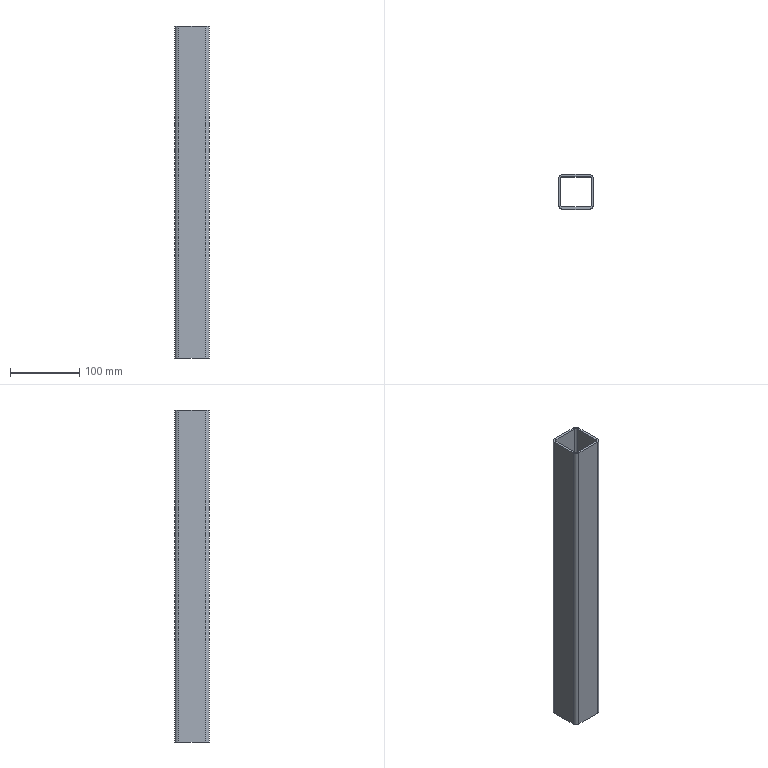Part | SolidWorks | features WeldMemberFeat 1, WeldmentFeature 1 | 1 solid | 18 faces | box 50 x 50 x 480 mm | volume 259595 mm3 | plane 10 | cylinder 8 | commonest cylinder face diameters 6 x4 12 x4
STEP:
#1=CARTESIAN_POINT('',(-25.,19.,0.));
#2=VERTEX_POINT('',#1);
#3=CARTESIAN_POINT('',(-19.,25.,0.));
#4=VERTEX_POINT('',#3);
#5=CARTESIAN_POINT('',(-19.,19.,0.));
#6=DIRECTION('',(0.,0.,-1.));
#7=DIRECTION('',(-1.,0.,0.));
#8=AXIS2_PLACEMENT_3D('',#5,#6,#7);
#9=CIRCLE('',#8,6.);
#10=EDGE_CURVE('',#2,#4,#9,.T.);
#11=ORIENTED_EDGE('',*,*,#10,.T.);
#12=CARTESIAN_POINT('',(-19.,25.,-480.));
#13=VERTEX_POINT('',#12);
#14=CARTESIAN_POINT('',(-19.,25.,-480.));
#15=DIRECTION('',(0.,0.,1.));
#16=VECTOR('',#15,1000.);
#17=LINE('',#14,#16);
#18=EDGE_CURVE('',#13,#4,#17,.T.);
#19=ORIENTED_EDGE('',*,*,#18,.F.);
#20=CARTESIAN_POINT('',(-25.,19.,-480.));
#21=VERTEX_POINT('',#20);
#22=CARTESIAN_POINT('',(-19.,19.,-480.));
#23=DIRECTION('',(0.,0.,-1.));
#24=DIRECTION('',(-1.,0.,0.));
#25=AXIS2_PLACEMENT_3D('',#22,#23,#24);
#26=CIRCLE('',#25,6.);
#27=EDGE_CURVE('',#21,#13,#26,.T.);
#28=ORIENTED_EDGE('',*,*,#27,.F.);
#29=CARTESIAN_POINT('',(-25.,19.,-480.));
#30=DIRECTION('',(0.,0.,1.));
#31=VECTOR('',#30,1000.);
#32=LINE('',#29,#31);
#33=EDGE_CURVE('',#21,#2,#32,.T.);
#34=ORIENTED_EDGE('',*,*,#33,.T.);
#35=EDGE_LOOP('',(#11,#19,#28,#34));
#36=FACE_OUTER_BOUND('',#35,.T.);
#37=CARTESIAN_POINT('',(-19.,19.,-480.));
#38=DIRECTION('',(0.,0.,1.));
#39=DIRECTION('',(1.,0.,0.));
#40=AXIS2_PLACEMENT_3D('',#37,#38,#39);
#41=CYLINDRICAL_SURFACE('',#40,6.);
#42=ADVANCED_FACE('',(#36),#41,.T.);
#43=CARTESIAN_POINT('',(19.,25.,0.));
#44=VERTEX_POINT('',#43);
#45=CARTESIAN_POINT('',(-19.,25.,0.));
#46=DIRECTION('',(1.,0.,0.));
#47=VECTOR('',#46,1000.);
#48=LINE('',#45,#47);
#49=EDGE_CURVE('',#4,#44,#48,.T.);
#50=ORIENTED_EDGE('',*,*,#49,.T.);
#51=CARTESIAN_POINT('',(19.,25.,-480.));
#52=VERTEX_POINT('',#51);
#53=CARTESIAN_POINT('',(19.,25.,-480.));
#54=DIRECTION('',(0.,0.,1.));
#55=VECTOR('',#54,1000.);
#56=LINE('',#53,#55);
#57=EDGE_CURVE('',#52,#44,#56,.T.);
#58=ORIENTED_EDGE('',*,*,#57,.F.);
#59=CARTESIAN_POINT('',(-19.,25.,-480.));
#60=DIRECTION('',(1.,0.,0.));
#61=VECTOR('',#60,1000.);
#62=LINE('',#59,#61);
#63=EDGE_CURVE('',#13,#52,#62,.T.);
#64=ORIENTED_EDGE('',*,*,#63,.F.);
#65=ORIENTED_EDGE('',*,*,#18,.T.);
#66=EDGE_LOOP('',(#50,#58,#64,#65));
#67=FACE_OUTER_BOUND('',#66,.T.);
#68=CARTESIAN_POINT('',(-19.,25.,-480.));
#69=DIRECTION('',(0.,-1.,0.));
#70=DIRECTION('',(0.,0.,-1.));
#71=AXIS2_PLACEMENT_3D('',#68,#69,#70);
#72=PLANE('',#71);
#73=ADVANCED_FACE('',(#67),#72,.F.);
#74=CARTESIAN_POINT('',(25.,19.,0.));
#75=VERTEX_POINT('',#74);
#76=CARTESIAN_POINT('',(19.,19.,0.));
#77=DIRECTION('',(0.,0.,-1.));
#78=DIRECTION('',(-1.,0.,0.));
#79=AXIS2_PLACEMENT_3D('',#76,#77,#78);
#80=CIRCLE('',#79,6.);
#81=EDGE_CURVE('',#44,#75,#80,.T.);
#82=ORIENTED_EDGE('',*,*,#81,.T.);
#83=CARTESIAN_POINT('',(25.,19.,-480.));
#84=VERTEX_POINT('',#83);
#85=CARTESIAN_POINT('',(25.,19.,-480.));
#86=DIRECTION('',(0.,0.,1.));
#87=VECTOR('',#86,1000.);
#88=LINE('',#85,#87);
#89=EDGE_CURVE('',#84,#75,#88,.T.);
#90=ORIENTED_EDGE('',*,*,#89,.F.);
#91=CARTESIAN_POINT('',(19.,19.,-480.));
#92=DIRECTION('',(0.,0.,-1.));
#93=DIRECTION('',(-1.,0.,0.));
#94=AXIS2_PLACEMENT_3D('',#91,#92,#93);
#95=CIRCLE('',#94,6.);
#96=EDGE_CURVE('',#52,#84,#95,.T.);
#97=ORIENTED_EDGE('',*,*,#96,.F.);
#98=ORIENTED_EDGE('',*,*,#57,.T.);
#99=EDGE_LOOP('',(#82,#90,#97,#98));
#100=FACE_OUTER_BOUND('',#99,.T.);
#101=CARTESIAN_POINT('',(19.,19.,-480.));
#102=DIRECTION('',(0.,0.,1.));
#103=DIRECTION('',(1.,0.,0.));
#104=AXIS2_PLACEMENT_3D('',#101,#102,#103);
#105=CYLINDRICAL_SURFACE('',#104,6.);
#106=ADVANCED_FACE('',(#100),#105,.T.);
#107=CARTESIAN_POINT('',(25.,-19.,0.));
#108=VERTEX_POINT('',#107);
#109=CARTESIAN_POINT('',(25.,-19.,0.));
#110=DIRECTION('',(0.,-1.,0.));
#111=VECTOR('',#110,1000.);
#112=LINE('',#109,#111);
#113=EDGE_CURVE('',#75,#108,#112,.T.);
#114=ORIENTED_EDGE('',*,*,#113,.T.);
#115=CARTESIAN_POINT('',(25.,-19.,-480.));
#116=VERTEX_POINT('',#115);
#117=CARTESIAN_POINT('',(25.,-19.,-480.));
#118=DIRECTION('',(0.,0.,1.));
#119=VECTOR('',#118,1000.);
#120=LINE('',#117,#119);
#121=EDGE_CURVE('',#116,#108,#120,.T.);
#122=ORIENTED_EDGE('',*,*,#121,.F.);
#123=CARTESIAN_POINT('',(25.,-19.,-480.));
#124=DIRECTION('',(0.,-1.,0.));
#125=VECTOR('',#124,1000.);
#126=LINE('',#123,#125);
#127=EDGE_CURVE('',#84,#116,#126,.T.);
#128=ORIENTED_EDGE('',*,*,#127,.F.);
#129=ORIENTED_EDGE('',*,*,#89,.T.);
#130=EDGE_LOOP('',(#114,#122,#128,#129));
#131=FACE_OUTER_BOUND('',#130,.T.);
#132=CARTESIAN_POINT('',(25.,-19.,-480.));
#133=DIRECTION('',(-1.,0.,0.));
#134=DIRECTION('',(0.,0.,1.));
#135=AXIS2_PLACEMENT_3D('',#132,#133,#134);
#136=PLANE('',#135);
#137=ADVANCED_FACE('',(#131),#136,.F.);
#138=CARTESIAN_POINT('',(19.,-25.,0.));
#139=VERTEX_POINT('',#138);
#140=CARTESIAN_POINT('',(19.,-19.,0.));
#141=DIRECTION('',(0.,0.,-1.));
#142=DIRECTION('',(-1.,0.,0.));
#143=AXIS2_PLACEMENT_3D('',#140,#141,#142);
#144=CIRCLE('',#143,6.);
#145=EDGE_CURVE('',#108,#139,#144,.T.);
#146=ORIENTED_EDGE('',*,*,#145,.T.);
#147=CARTESIAN_POINT('',(19.,-25.,-480.));
#148=VERTEX_POINT('',#147);
#149=CARTESIAN_POINT('',(19.,-25.,-480.));
#150=DIRECTION('',(0.,0.,1.));
#151=VECTOR('',#150,1000.);
#152=LINE('',#149,#151);
#153=EDGE_CURVE('',#148,#139,#152,.T.);
#154=ORIENTED_EDGE('',*,*,#153,.F.);
#155=CARTESIAN_POINT('',(19.,-19.,-480.));
#156=DIRECTION('',(0.,0.,-1.));
#157=DIRECTION('',(-1.,0.,0.));
#158=AXIS2_PLACEMENT_3D('',#155,#156,#157);
#159=CIRCLE('',#158,6.);
#160=EDGE_CURVE('',#116,#148,#159,.T.);
#161=ORIENTED_EDGE('',*,*,#160,.F.);
#162=ORIENTED_EDGE('',*,*,#121,.T.);
#163=EDGE_LOOP('',(#146,#154,#161,#162));
#164=FACE_OUTER_BOUND('',#163,.T.);
#165=CARTESIAN_POINT('',(19.,-19.,-480.));
#166=DIRECTION('',(0.,0.,1.));
#167=DIRECTION('',(1.,0.,0.));
#168=AXIS2_PLACEMENT_3D('',#165,#166,#167);
#169=CYLINDRICAL_SURFACE('',#168,6.);
#170=ADVANCED_FACE('',(#164),#169,.T.);
#171=CARTESIAN_POINT('',(-19.,-25.,0.));
#172=VERTEX_POINT('',#171);
#173=CARTESIAN_POINT('',(19.,-25.,0.));
#174=DIRECTION('',(-1.,0.,0.));
#175=VECTOR('',#174,1000.);
#176=LINE('',#173,#175);
#177=EDGE_CURVE('',#139,#172,#176,.T.);
#178=ORIENTED_EDGE('',*,*,#177,.T.);
#179=CARTESIAN_POINT('',(-19.,-25.,-480.));
#180=VERTEX_POINT('',#179);
#181=CARTESIAN_POINT('',(-19.,-25.,-480.));
#182=DIRECTION('',(0.,0.,1.));
#183=VECTOR('',#182,1000.);
#184=LINE('',#181,#183);
#185=EDGE_CURVE('',#180,#172,#184,.T.);
#186=ORIENTED_EDGE('',*,*,#185,.F.);
#187=CARTESIAN_POINT('',(19.,-25.,-480.));
#188=DIRECTION('',(-1.,0.,0.));
#189=VECTOR('',#188,1000.);
#190=LINE('',#187,#189);
#191=EDGE_CURVE('',#148,#180,#190,.T.);
#192=ORIENTED_EDGE('',*,*,#191,.F.);
#193=ORIENTED_EDGE('',*,*,#153,.T.);
#194=EDGE_LOOP('',(#178,#186,#192,#193));
#195=FACE_OUTER_BOUND('',#194,.T.);
#196=CARTESIAN_POINT('',(19.,-25.,-480.));
#197=DIRECTION('',(0.,1.,0.));
#198=DIRECTION('',(0.,0.,1.));
#199=AXIS2_PLACEMENT_3D('',#196,#197,#198);
#200=PLANE('',#199);
#201=ADVANCED_FACE('',(#195),#200,.F.);
#202=CARTESIAN_POINT('',(-25.,-19.,0.));
#203=VERTEX_POINT('',#202);
#204=CARTESIAN_POINT('',(-19.,-19.,0.));
#205=DIRECTION('',(0.,0.,-1.));
#206=DIRECTION('',(-1.,0.,0.));
#207=AXIS2_PLACEMENT_3D('',#204,#205,#206);
#208=CIRCLE('',#207,6.);
#209=EDGE_CURVE('',#172,#203,#208,.T.);
#210=ORIENTED_EDGE('',*,*,#209,.T.);
#211=CARTESIAN_POINT('',(-25.,-19.,-480.));
#212=VERTEX_POINT('',#211);
#213=CARTESIAN_POINT('',(-25.,-19.,-480.));
#214=DIRECTION('',(0.,0.,1.));
#215=VECTOR('',#214,1000.);
#216=LINE('',#213,#215);
#217=EDGE_CURVE('',#212,#203,#216,.T.);
#218=ORIENTED_EDGE('',*,*,#217,.F.);
#219=CARTESIAN_POINT('',(-19.,-19.,-480.));
#220=DIRECTION('',(0.,0.,-1.));
#221=DIRECTION('',(-1.,0.,0.));
#222=AXIS2_PLACEMENT_3D('',#219,#220,#221);
#223=CIRCLE('',#222,6.);
#224=EDGE_CURVE('',#180,#212,#223,.T.);
#225=ORIENTED_EDGE('',*,*,#224,.F.);
#226=ORIENTED_EDGE('',*,*,#185,.T.);
#227=EDGE_LOOP('',(#210,#218,#225,#226));
#228=FACE_OUTER_BOUND('',#227,.T.);
#229=CARTESIAN_POINT('',(-19.,-19.,-480.));
#230=DIRECTION('',(0.,0.,1.));
#231=DIRECTION('',(1.,0.,0.));
#232=AXIS2_PLACEMENT_3D('',#229,#230,#231);
#233=CYLINDRICAL_SURFACE('',#232,6.);
#234=ADVANCED_FACE('',(#228),#233,.T.);
#235=CARTESIAN_POINT('',(19.,22.,0.));
#236=VERTEX_POINT('',#235);
#237=CARTESIAN_POINT('',(22.,19.,0.));
#238=VERTEX_POINT('',#237);
#239=CARTESIAN_POINT('',(19.,19.,0.));
#240=DIRECTION('',(0.,0.,-1.));
#241=DIRECTION('',(-1.,0.,0.));
#242=AXIS2_PLACEMENT_3D('',#239,#240,#241);
#243=CIRCLE('',#242,3.);
#244=EDGE_CURVE('',#236,#238,#243,.T.);
#245=ORIENTED_EDGE('',*,*,#244,.F.);
#246=CARTESIAN_POINT('',(19.,22.,-480.));
#247=VERTEX_POINT('',#246);
#248=CARTESIAN_POINT('',(19.,22.,-480.));
#249=DIRECTION('',(0.,0.,1.));
#250=VECTOR('',#249,1000.);
#251=LINE('',#248,#250);
#252=EDGE_CURVE('',#247,#236,#251,.T.);
#253=ORIENTED_EDGE('',*,*,#252,.F.);
#254=CARTESIAN_POINT('',(22.,19.,-480.));
#255=VERTEX_POINT('',#254);
#256=CARTESIAN_POINT('',(19.,19.,-480.));
#257=DIRECTION('',(0.,0.,-1.));
#258=DIRECTION('',(-1.,0.,0.));
#259=AXIS2_PLACEMENT_3D('',#256,#257,#258);
#260=CIRCLE('',#259,3.);
#261=EDGE_CURVE('',#247,#255,#260,.T.);
#262=ORIENTED_EDGE('',*,*,#261,.T.);
#263=CARTESIAN_POINT('',(22.,19.,-480.));
#264=DIRECTION('',(0.,0.,1.));
#265=VECTOR('',#264,1000.);
#266=LINE('',#263,#265);
#267=EDGE_CURVE('',#255,#238,#266,.T.);
#268=ORIENTED_EDGE('',*,*,#267,.T.);
#269=EDGE_LOOP('',(#245,#253,#262,#268));
#270=FACE_OUTER_BOUND('',#269,.T.);
#271=CARTESIAN_POINT('',(19.,19.,-480.));
#272=DIRECTION('',(0.,0.,1.));
#273=DIRECTION('',(1.,0.,0.));
#274=AXIS2_PLACEMENT_3D('',#271,#272,#273);
#275=CYLINDRICAL_SURFACE('',#274,3.);
#276=ADVANCED_FACE('',(#270),#275,.F.);
#277=CARTESIAN_POINT('',(-19.,22.,0.));
#278=VERTEX_POINT('',#277);
#279=CARTESIAN_POINT('',(-19.,22.,0.));
#280=DIRECTION('',(1.,0.,0.));
#281=VECTOR('',#280,1000.);
#282=LINE('',#279,#281);
#283=EDGE_CURVE('',#278,#236,#282,.T.);
#284=ORIENTED_EDGE('',*,*,#283,.F.);
#285=CARTESIAN_POINT('',(-19.,22.,-480.));
#286=VERTEX_POINT('',#285);
#287=CARTESIAN_POINT('',(-19.,22.,-480.));
#288=DIRECTION('',(0.,0.,1.));
#289=VECTOR('',#288,1000.);
#290=LINE('',#287,#289);
#291=EDGE_CURVE('',#286,#278,#290,.T.);
#292=ORIENTED_EDGE('',*,*,#291,.F.);
#293=CARTESIAN_POINT('',(-19.,22.,-480.));
#294=DIRECTION('',(1.,0.,0.));
#295=VECTOR('',#294,1000.);
#296=LINE('',#293,#295);
#297=EDGE_CURVE('',#286,#247,#296,.T.);
#298=ORIENTED_EDGE('',*,*,#297,.T.);
#299=ORIENTED_EDGE('',*,*,#252,.T.);
#300=EDGE_LOOP('',(#284,#292,#298,#299));
#301=FACE_OUTER_BOUND('',#300,.T.);
#302=CARTESIAN_POINT('',(-19.,22.,-480.));
#303=DIRECTION('',(0.,-1.,0.));
#304=DIRECTION('',(0.,0.,-1.));
#305=AXIS2_PLACEMENT_3D('',#302,#303,#304);
#306=PLANE('',#305);
#307=ADVANCED_FACE('',(#301),#306,.T.);
#308=CARTESIAN_POINT('',(-22.,19.,0.));
#309=VERTEX_POINT('',#308);
#310=CARTESIAN_POINT('',(-19.,19.,0.));
#311=DIRECTION('',(0.,0.,-1.));
#312=DIRECTION('',(-1.,0.,0.));
#313=AXIS2_PLACEMENT_3D('',#310,#311,#312);
#314=CIRCLE('',#313,3.);
#315=EDGE_CURVE('',#309,#278,#314,.T.);
#316=ORIENTED_EDGE('',*,*,#315,.F.);
#317=CARTESIAN_POINT('',(-22.,19.,-480.));
#318=VERTEX_POINT('',#317);
#319=CARTESIAN_POINT('',(-22.,19.,-480.));
#320=DIRECTION('',(0.,0.,1.));
#321=VECTOR('',#320,1000.);
#322=LINE('',#319,#321);
#323=EDGE_CURVE('',#318,#309,#322,.T.);
#324=ORIENTED_EDGE('',*,*,#323,.F.);
#325=CARTESIAN_POINT('',(-19.,19.,-480.));
#326=DIRECTION('',(0.,0.,-1.));
#327=DIRECTION('',(-1.,0.,0.));
#328=AXIS2_PLACEMENT_3D('',#325,#326,#327);
#329=CIRCLE('',#328,3.);
#330=EDGE_CURVE('',#318,#286,#329,.T.);
#331=ORIENTED_EDGE('',*,*,#330,.T.);
#332=ORIENTED_EDGE('',*,*,#291,.T.);
#333=EDGE_LOOP('',(#316,#324,#331,#332));
#334=FACE_OUTER_BOUND('',#333,.T.);
#335=CARTESIAN_POINT('',(-19.,19.,-480.));
#336=DIRECTION('',(0.,0.,1.));
#337=DIRECTION('',(1.,0.,0.));
#338=AXIS2_PLACEMENT_3D('',#335,#336,#337);
#339=CYLINDRICAL_SURFACE('',#338,3.);
#340=ADVANCED_FACE('',(#334),#339,.F.);
#341=CARTESIAN_POINT('',(-22.,-19.,0.));
#342=VERTEX_POINT('',#341);
#343=CARTESIAN_POINT('',(-22.,19.,0.));
#344=DIRECTION('',(0.,1.,0.));
#345=VECTOR('',#344,1000.);
#346=LINE('',#343,#345);
#347=EDGE_CURVE('',#342,#309,#346,.T.);
#348=ORIENTED_EDGE('',*,*,#347,.F.);
#349=CARTESIAN_POINT('',(-22.,-19.,-480.));
#350=VERTEX_POINT('',#349);
#351=CARTESIAN_POINT('',(-22.,-19.,-480.));
#352=DIRECTION('',(0.,0.,1.));
#353=VECTOR('',#352,1000.);
#354=LINE('',#351,#353);
#355=EDGE_CURVE('',#350,#342,#354,.T.);
#356=ORIENTED_EDGE('',*,*,#355,.F.);
#357=CARTESIAN_POINT('',(-22.,19.,-480.));
#358=DIRECTION('',(0.,1.,0.));
#359=VECTOR('',#358,1000.);
#360=LINE('',#357,#359);
#361=EDGE_CURVE('',#350,#318,#360,.T.);
#362=ORIENTED_EDGE('',*,*,#361,.T.);
#363=ORIENTED_EDGE('',*,*,#323,.T.);
#364=EDGE_LOOP('',(#348,#356,#362,#363));
#365=FACE_OUTER_BOUND('',#364,.T.);
#366=CARTESIAN_POINT('',(-22.,19.,-480.));
#367=DIRECTION('',(1.,0.,0.));
#368=DIRECTION('',(0.,0.,-1.));
#369=AXIS2_PLACEMENT_3D('',#366,#367,#368);
#370=PLANE('',#369);
#371=ADVANCED_FACE('',(#365),#370,.T.);
#372=CARTESIAN_POINT('',(-19.,-22.,0.));
#373=VERTEX_POINT('',#372);
#374=CARTESIAN_POINT('',(-19.,-19.,0.));
#375=DIRECTION('',(0.,0.,-1.));
#376=DIRECTION('',(-1.,0.,0.));
#377=AXIS2_PLACEMENT_3D('',#374,#375,#376);
#378=CIRCLE('',#377,3.);
#379=EDGE_CURVE('',#373,#342,#378,.T.);
#380=ORIENTED_EDGE('',*,*,#379,.F.);
#381=CARTESIAN_POINT('',(-19.,-22.,-480.));
#382=VERTEX_POINT('',#381);
#383=CARTESIAN_POINT('',(-19.,-22.,-480.));
#384=DIRECTION('',(0.,0.,1.));
#385=VECTOR('',#384,1000.);
#386=LINE('',#383,#385);
#387=EDGE_CURVE('',#382,#373,#386,.T.);
#388=ORIENTED_EDGE('',*,*,#387,.F.);
#389=CARTESIAN_POINT('',(-19.,-19.,-480.));
#390=DIRECTION('',(0.,0.,-1.));
#391=DIRECTION('',(-1.,0.,0.));
#392=AXIS2_PLACEMENT_3D('',#389,#390,#391);
#393=CIRCLE('',#392,3.);
#394=EDGE_CURVE('',#382,#350,#393,.T.);
#395=ORIENTED_EDGE('',*,*,#394,.T.);
#396=ORIENTED_EDGE('',*,*,#355,.T.);
#397=EDGE_LOOP('',(#380,#388,#395,#396));
#398=FACE_OUTER_BOUND('',#397,.T.);
#399=CARTESIAN_POINT('',(-19.,-19.,-480.));
#400=DIRECTION('',(0.,0.,1.));
#401=DIRECTION('',(1.,0.,0.));
#402=AXIS2_PLACEMENT_3D('',#399,#400,#401);
#403=CYLINDRICAL_SURFACE('',#402,3.);
#404=ADVANCED_FACE('',(#398),#403,.F.);
#405=CARTESIAN_POINT('',(19.,-22.,0.));
#406=VERTEX_POINT('',#405);
#407=CARTESIAN_POINT('',(19.,-22.,0.));
#408=DIRECTION('',(-1.,0.,0.));
#409=VECTOR('',#408,1000.);
#410=LINE('',#407,#409);
#411=EDGE_CURVE('',#406,#373,#410,.T.);
#412=ORIENTED_EDGE('',*,*,#411,.F.);
#413=CARTESIAN_POINT('',(19.,-22.,-480.));
#414=VERTEX_POINT('',#413);
#415=CARTESIAN_POINT('',(19.,-22.,-480.));
#416=DIRECTION('',(0.,0.,1.));
#417=VECTOR('',#416,1000.);
#418=LINE('',#415,#417);
#419=EDGE_CURVE('',#414,#406,#418,.T.);
#420=ORIENTED_EDGE('',*,*,#419,.F.);
#421=CARTESIAN_POINT('',(19.,-22.,-480.));
#422=DIRECTION('',(-1.,0.,0.));
#423=VECTOR('',#422,1000.);
#424=LINE('',#421,#423);
#425=EDGE_CURVE('',#414,#382,#424,.T.);
#426=ORIENTED_EDGE('',*,*,#425,.T.);
#427=ORIENTED_EDGE('',*,*,#387,.T.);
#428=EDGE_LOOP('',(#412,#420,#426,#427));
#429=FACE_OUTER_BOUND('',#428,.T.);
#430=CARTESIAN_POINT('',(19.,-22.,-480.));
#431=DIRECTION('',(0.,1.,0.));
#432=DIRECTION('',(0.,0.,1.));
#433=AXIS2_PLACEMENT_3D('',#430,#431,#432);
#434=PLANE('',#433);
#435=ADVANCED_FACE('',(#429),#434,.T.);
#436=CARTESIAN_POINT('',(22.,-19.,0.));
#437=VERTEX_POINT('',#436);
#438=CARTESIAN_POINT('',(19.,-19.,0.));
#439=DIRECTION('',(0.,0.,-1.));
#440=DIRECTION('',(-1.,0.,0.));
#441=AXIS2_PLACEMENT_3D('',#438,#439,#440);
#442=CIRCLE('',#441,3.);
#443=EDGE_CURVE('',#437,#406,#442,.T.);
#444=ORIENTED_EDGE('',*,*,#443,.F.);
#445=CARTESIAN_POINT('',(22.,-19.,-480.));
#446=VERTEX_POINT('',#445);
#447=CARTESIAN_POINT('',(22.,-19.,-480.));
#448=DIRECTION('',(0.,0.,1.));
#449=VECTOR('',#448,1000.);
#450=LINE('',#447,#449);
#451=EDGE_CURVE('',#446,#437,#450,.T.);
#452=ORIENTED_EDGE('',*,*,#451,.F.);
#453=CARTESIAN_POINT('',(19.,-19.,-480.));
#454=DIRECTION('',(0.,0.,-1.));
#455=DIRECTION('',(-1.,0.,0.));
#456=AXIS2_PLACEMENT_3D('',#453,#454,#455);
#457=CIRCLE('',#456,3.);
#458=EDGE_CURVE('',#446,#414,#457,.T.);
#459=ORIENTED_EDGE('',*,*,#458,.T.);
#460=ORIENTED_EDGE('',*,*,#419,.T.);
#461=EDGE_LOOP('',(#444,#452,#459,#460));
#462=FACE_OUTER_BOUND('',#461,.T.);
#463=CARTESIAN_POINT('',(19.,-19.,-480.));
#464=DIRECTION('',(0.,0.,1.));
#465=DIRECTION('',(1.,0.,0.));
#466=AXIS2_PLACEMENT_3D('',#463,#464,#465);
#467=CYLINDRICAL_SURFACE('',#466,3.);
#468=ADVANCED_FACE('',(#462),#467,.F.);
#469=CARTESIAN_POINT('',(22.,-19.,0.));
#470=DIRECTION('',(0.,-1.,0.));
#471=VECTOR('',#470,1000.);
#472=LINE('',#469,#471);
#473=EDGE_CURVE('',#238,#437,#472,.T.);
#474=ORIENTED_EDGE('',*,*,#473,.F.);
#475=ORIENTED_EDGE('',*,*,#267,.F.);
#476=CARTESIAN_POINT('',(22.,-19.,-480.));
#477=DIRECTION('',(0.,-1.,0.));
#478=VECTOR('',#477,1000.);
#479=LINE('',#476,#478);
#480=EDGE_CURVE('',#255,#446,#479,.T.);
#481=ORIENTED_EDGE('',*,*,#480,.T.);
#482=ORIENTED_EDGE('',*,*,#451,.T.);
#483=EDGE_LOOP('',(#474,#475,#481,#482));
#484=FACE_OUTER_BOUND('',#483,.T.);
#485=CARTESIAN_POINT('',(22.,-19.,-480.));
#486=DIRECTION('',(-1.,0.,0.));
#487=DIRECTION('',(0.,0.,1.));
#488=AXIS2_PLACEMENT_3D('',#485,#486,#487);
#489=PLANE('',#488);
#490=ADVANCED_FACE('',(#484),#489,.T.);
#491=CARTESIAN_POINT('',(-25.,19.,0.));
#492=DIRECTION('',(0.,1.,0.));
#493=VECTOR('',#492,1000.);
#494=LINE('',#491,#493);
#495=EDGE_CURVE('',#203,#2,#494,.T.);
#496=ORIENTED_EDGE('',*,*,#495,.T.);
#497=ORIENTED_EDGE('',*,*,#33,.F.);
#498=CARTESIAN_POINT('',(-25.,19.,-480.));
#499=DIRECTION('',(0.,1.,0.));
#500=VECTOR('',#499,1000.);
#501=LINE('',#498,#500);
#502=EDGE_CURVE('',#212,#21,#501,.T.);
#503=ORIENTED_EDGE('',*,*,#502,.F.);
#504=ORIENTED_EDGE('',*,*,#217,.T.);
#505=EDGE_LOOP('',(#496,#497,#503,#504));
#506=FACE_OUTER_BOUND('',#505,.T.);
#507=CARTESIAN_POINT('',(-25.,19.,-480.));
#508=DIRECTION('',(1.,0.,0.));
#509=DIRECTION('',(0.,0.,-1.));
#510=AXIS2_PLACEMENT_3D('',#507,#508,#509);
#511=PLANE('',#510);
#512=ADVANCED_FACE('',(#506),#511,.F.);
#513=ORIENTED_EDGE('',*,*,#261,.F.);
#514=ORIENTED_EDGE('',*,*,#297,.F.);
#515=ORIENTED_EDGE('',*,*,#330,.F.);
#516=ORIENTED_EDGE('',*,*,#361,.F.);
#517=ORIENTED_EDGE('',*,*,#394,.F.);
#518=ORIENTED_EDGE('',*,*,#425,.F.);
#519=ORIENTED_EDGE('',*,*,#458,.F.);
#520=ORIENTED_EDGE('',*,*,#480,.F.);
#521=EDGE_LOOP('',(#513,#514,#515,#516,#517,#518,#519,#520));
#522=FACE_BOUND('',#521,.T.);
#523=ORIENTED_EDGE('',*,*,#27,.T.);
#524=ORIENTED_EDGE('',*,*,#63,.T.);
#525=ORIENTED_EDGE('',*,*,#96,.T.);
#526=ORIENTED_EDGE('',*,*,#127,.T.);
#527=ORIENTED_EDGE('',*,*,#160,.T.);
#528=ORIENTED_EDGE('',*,*,#191,.T.);
#529=ORIENTED_EDGE('',*,*,#224,.T.);
#530=ORIENTED_EDGE('',*,*,#502,.T.);
#531=EDGE_LOOP('',(#523,#524,#525,#526,#527,#528,#529,#530));
#532=FACE_OUTER_BOUND('',#531,.T.);
#533=CARTESIAN_POINT('',(-19.,19.,-480.));
#534=DIRECTION('',(0.,0.,-1.));
#535=DIRECTION('',(-1.,0.,0.));
#536=AXIS2_PLACEMENT_3D('',#533,#534,#535);
#537=PLANE('',#536);
#538=ADVANCED_FACE('',(#522,#532),#537,.T.);
#539=ORIENTED_EDGE('',*,*,#244,.T.);
#540=ORIENTED_EDGE('',*,*,#473,.T.);
#541=ORIENTED_EDGE('',*,*,#443,.T.);
#542=ORIENTED_EDGE('',*,*,#411,.T.);
#543=ORIENTED_EDGE('',*,*,#379,.T.);
#544=ORIENTED_EDGE('',*,*,#347,.T.);
#545=ORIENTED_EDGE('',*,*,#315,.T.);
#546=ORIENTED_EDGE('',*,*,#283,.T.);
#547=EDGE_LOOP('',(#539,#540,#541,#542,#543,#544,#545,#546));
#548=FACE_BOUND('',#547,.T.);
#549=ORIENTED_EDGE('',*,*,#10,.F.);
#550=ORIENTED_EDGE('',*,*,#495,.F.);
#551=ORIENTED_EDGE('',*,*,#209,.F.);
#552=ORIENTED_EDGE('',*,*,#177,.F.);
#553=ORIENTED_EDGE('',*,*,#145,.F.);
#554=ORIENTED_EDGE('',*,*,#113,.F.);
#555=ORIENTED_EDGE('',*,*,#81,.F.);
#556=ORIENTED_EDGE('',*,*,#49,.F.);
#557=EDGE_LOOP('',(#549,#550,#551,#552,#553,#554,#555,#556));
#558=FACE_OUTER_BOUND('',#557,.T.);
#559=CARTESIAN_POINT('',(-19.,19.,0.));
#560=DIRECTION('',(0.,0.,-1.));
#561=DIRECTION('',(-1.,0.,0.));
#562=AXIS2_PLACEMENT_3D('',#559,#560,#561);
#563=PLANE('',#562);
#564=ADVANCED_FACE('',(#548,#558),#563,.F.);
#565=CLOSED_SHELL('',(#42,#73,#106,#137,#170,#201,#234,#276,#307,#340,#371,#404,#435,#468,#490,#512,#538,#564));
#566=MANIFOLD_SOLID_BREP('',#565);
#567=CARTESIAN_POINT('',(0.,0.,0.));
#568=DIRECTION('',(0.,0.,1.));
#569=DIRECTION('',(1.,0.,0.));
#570=AXIS2_PLACEMENT_3D('',#567,#568,#569);
#571=(LENGTH_UNIT()NAMED_UNIT(*)SI_UNIT(.MILLI.,.METRE.));
#572=UNCERTAINTY_MEASURE_WITH_UNIT(LENGTH_MEASURE(0.00001),#571,'','');
#573=(NAMED_UNIT(*)PLANE_ANGLE_UNIT()SI_UNIT($,.RADIAN.));
#574=(NAMED_UNIT(*)SI_UNIT($,.STERADIAN.)SOLID_ANGLE_UNIT());
#575=(GEOMETRIC_REPRESENTATION_CONTEXT(3)GLOBAL_UNCERTAINTY_ASSIGNED_CONTEXT((#572))GLOBAL_UNIT_ASSIGNED_CONTEXT((#571,#573,#574))REPRESENTATION_CONTEXT('',''));
#576=ADVANCED_BREP_SHAPE_REPRESENTATION('',(#566,#570),#575);